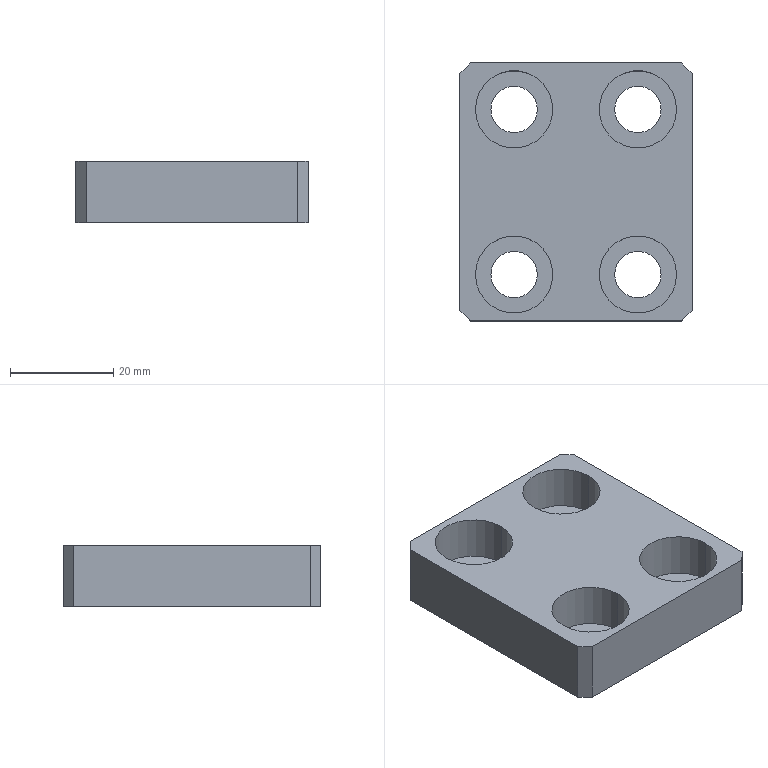Part | SolidWorks | features Chamfer 1, Extrusion 1, HoleWzd 1 | 1 solid | 30 faces | box 45 x 50 x 12 mm | volume 19960 mm3 | cylinder 16 | plane 14 | commonest cylinder face diameters 9 x8 15 x8
STEP:
#1=CARTESIAN_POINT('',(-19.5,16.,3.4));
#2=VERTEX_POINT('',#1);
#3=CARTESIAN_POINT('',(-4.5,16.,3.4));
#4=VERTEX_POINT('',#3);
#5=CARTESIAN_POINT('',(-12.,16.,3.4));
#6=DIRECTION('',(0.,0.,1.));
#7=DIRECTION('',(1.,0.,0.));
#8=AXIS2_PLACEMENT_3D('',#5,#6,#7);
#9=CIRCLE('',#8,7.5);
#10=EDGE_CURVE('',#2,#4,#9,.T.);
#11=ORIENTED_EDGE('',*,*,#10,.F.);
#12=CARTESIAN_POINT('',(-19.5,16.,12.));
#13=VERTEX_POINT('',#12);
#14=CARTESIAN_POINT('',(-19.5,16.,12.));
#15=DIRECTION('',(0.,0.,1.));
#16=VECTOR('',#15,1000.);
#17=LINE('',#14,#16);
#18=EDGE_CURVE('',#2,#13,#17,.T.);
#19=ORIENTED_EDGE('',*,*,#18,.T.);
#20=CARTESIAN_POINT('',(-4.5,16.,12.));
#21=VERTEX_POINT('',#20);
#22=CARTESIAN_POINT('',(-12.,16.,12.));
#23=DIRECTION('',(0.,0.,1.));
#24=DIRECTION('',(1.,0.,0.));
#25=AXIS2_PLACEMENT_3D('',#22,#23,#24);
#26=CIRCLE('',#25,7.5);
#27=EDGE_CURVE('',#13,#21,#26,.T.);
#28=ORIENTED_EDGE('',*,*,#27,.T.);
#29=CARTESIAN_POINT('',(-4.5,16.,12.));
#30=DIRECTION('',(0.,0.,1.));
#31=VECTOR('',#30,1000.);
#32=LINE('',#29,#31);
#33=EDGE_CURVE('',#4,#21,#32,.T.);
#34=ORIENTED_EDGE('',*,*,#33,.F.);
#35=EDGE_LOOP('',(#11,#19,#28,#34));
#36=FACE_OUTER_BOUND('',#35,.T.);
#37=CARTESIAN_POINT('',(-12.,16.,12.));
#38=DIRECTION('',(0.,0.,1.));
#39=DIRECTION('',(1.,0.,0.));
#40=AXIS2_PLACEMENT_3D('',#37,#38,#39);
#41=CYLINDRICAL_SURFACE('',#40,7.5);
#42=ADVANCED_FACE('',(#36),#41,.F.);
#43=CARTESIAN_POINT('',(-16.5,16.,0.));
#44=VERTEX_POINT('',#43);
#45=CARTESIAN_POINT('',(-7.5,16.,0.));
#46=VERTEX_POINT('',#45);
#47=CARTESIAN_POINT('',(-12.,16.,0.));
#48=DIRECTION('',(0.,0.,1.));
#49=DIRECTION('',(1.,0.,0.));
#50=AXIS2_PLACEMENT_3D('',#47,#48,#49);
#51=CIRCLE('',#50,4.5);
#52=EDGE_CURVE('',#44,#46,#51,.T.);
#53=ORIENTED_EDGE('',*,*,#52,.F.);
#54=CARTESIAN_POINT('',(-16.5,16.,3.4));
#55=VERTEX_POINT('',#54);
#56=CARTESIAN_POINT('',(-16.5,16.,12.));
#57=DIRECTION('',(0.,0.,1.));
#58=VECTOR('',#57,1000.);
#59=LINE('',#56,#58);
#60=EDGE_CURVE('',#44,#55,#59,.T.);
#61=ORIENTED_EDGE('',*,*,#60,.T.);
#62=CARTESIAN_POINT('',(-7.5,16.,3.4));
#63=VERTEX_POINT('',#62);
#64=CARTESIAN_POINT('',(-12.,16.,3.4));
#65=DIRECTION('',(0.,0.,1.));
#66=DIRECTION('',(1.,0.,0.));
#67=AXIS2_PLACEMENT_3D('',#64,#65,#66);
#68=CIRCLE('',#67,4.5);
#69=EDGE_CURVE('',#55,#63,#68,.T.);
#70=ORIENTED_EDGE('',*,*,#69,.T.);
#71=CARTESIAN_POINT('',(-7.5,16.,12.));
#72=DIRECTION('',(0.,0.,1.));
#73=VECTOR('',#72,1000.);
#74=LINE('',#71,#73);
#75=EDGE_CURVE('',#46,#63,#74,.T.);
#76=ORIENTED_EDGE('',*,*,#75,.F.);
#77=EDGE_LOOP('',(#53,#61,#70,#76));
#78=FACE_OUTER_BOUND('',#77,.T.);
#79=CARTESIAN_POINT('',(-12.,16.,12.));
#80=DIRECTION('',(0.,0.,1.));
#81=DIRECTION('',(1.,0.,0.));
#82=AXIS2_PLACEMENT_3D('',#79,#80,#81);
#83=CYLINDRICAL_SURFACE('',#82,4.5);
#84=ADVANCED_FACE('',(#78),#83,.F.);
#85=CARTESIAN_POINT('',(4.5,16.,3.4));
#86=VERTEX_POINT('',#85);
#87=CARTESIAN_POINT('',(19.5,16.,3.4));
#88=VERTEX_POINT('',#87);
#89=CARTESIAN_POINT('',(12.,16.,3.4));
#90=DIRECTION('',(0.,0.,1.));
#91=DIRECTION('',(1.,0.,0.));
#92=AXIS2_PLACEMENT_3D('',#89,#90,#91);
#93=CIRCLE('',#92,7.5);
#94=EDGE_CURVE('',#86,#88,#93,.T.);
#95=ORIENTED_EDGE('',*,*,#94,.F.);
#96=CARTESIAN_POINT('',(4.5,16.,12.));
#97=VERTEX_POINT('',#96);
#98=CARTESIAN_POINT('',(4.5,16.,12.));
#99=DIRECTION('',(0.,0.,1.));
#100=VECTOR('',#99,1000.);
#101=LINE('',#98,#100);
#102=EDGE_CURVE('',#86,#97,#101,.T.);
#103=ORIENTED_EDGE('',*,*,#102,.T.);
#104=CARTESIAN_POINT('',(19.5,16.,12.));
#105=VERTEX_POINT('',#104);
#106=CARTESIAN_POINT('',(12.,16.,12.));
#107=DIRECTION('',(0.,0.,1.));
#108=DIRECTION('',(1.,0.,0.));
#109=AXIS2_PLACEMENT_3D('',#106,#107,#108);
#110=CIRCLE('',#109,7.5);
#111=EDGE_CURVE('',#97,#105,#110,.T.);
#112=ORIENTED_EDGE('',*,*,#111,.T.);
#113=CARTESIAN_POINT('',(19.5,16.,12.));
#114=DIRECTION('',(0.,0.,1.));
#115=VECTOR('',#114,1000.);
#116=LINE('',#113,#115);
#117=EDGE_CURVE('',#88,#105,#116,.T.);
#118=ORIENTED_EDGE('',*,*,#117,.F.);
#119=EDGE_LOOP('',(#95,#103,#112,#118));
#120=FACE_OUTER_BOUND('',#119,.T.);
#121=CARTESIAN_POINT('',(12.,16.,12.));
#122=DIRECTION('',(0.,0.,1.));
#123=DIRECTION('',(1.,0.,0.));
#124=AXIS2_PLACEMENT_3D('',#121,#122,#123);
#125=CYLINDRICAL_SURFACE('',#124,7.5);
#126=ADVANCED_FACE('',(#120),#125,.F.);
#127=CARTESIAN_POINT('',(7.5,16.,0.));
#128=VERTEX_POINT('',#127);
#129=CARTESIAN_POINT('',(16.5,16.,0.));
#130=VERTEX_POINT('',#129);
#131=CARTESIAN_POINT('',(12.,16.,0.));
#132=DIRECTION('',(0.,0.,1.));
#133=DIRECTION('',(1.,0.,0.));
#134=AXIS2_PLACEMENT_3D('',#131,#132,#133);
#135=CIRCLE('',#134,4.5);
#136=EDGE_CURVE('',#128,#130,#135,.T.);
#137=ORIENTED_EDGE('',*,*,#136,.F.);
#138=CARTESIAN_POINT('',(7.5,16.,3.4));
#139=VERTEX_POINT('',#138);
#140=CARTESIAN_POINT('',(7.5,16.,12.));
#141=DIRECTION('',(0.,0.,1.));
#142=VECTOR('',#141,1000.);
#143=LINE('',#140,#142);
#144=EDGE_CURVE('',#128,#139,#143,.T.);
#145=ORIENTED_EDGE('',*,*,#144,.T.);
#146=CARTESIAN_POINT('',(16.5,16.,3.4));
#147=VERTEX_POINT('',#146);
#148=CARTESIAN_POINT('',(12.,16.,3.4));
#149=DIRECTION('',(0.,0.,1.));
#150=DIRECTION('',(1.,0.,0.));
#151=AXIS2_PLACEMENT_3D('',#148,#149,#150);
#152=CIRCLE('',#151,4.5);
#153=EDGE_CURVE('',#139,#147,#152,.T.);
#154=ORIENTED_EDGE('',*,*,#153,.T.);
#155=CARTESIAN_POINT('',(16.5,16.,12.));
#156=DIRECTION('',(0.,0.,1.));
#157=VECTOR('',#156,1000.);
#158=LINE('',#155,#157);
#159=EDGE_CURVE('',#130,#147,#158,.T.);
#160=ORIENTED_EDGE('',*,*,#159,.F.);
#161=EDGE_LOOP('',(#137,#145,#154,#160));
#162=FACE_OUTER_BOUND('',#161,.T.);
#163=CARTESIAN_POINT('',(12.,16.,12.));
#164=DIRECTION('',(0.,0.,1.));
#165=DIRECTION('',(1.,0.,0.));
#166=AXIS2_PLACEMENT_3D('',#163,#164,#165);
#167=CYLINDRICAL_SURFACE('',#166,4.5);
#168=ADVANCED_FACE('',(#162),#167,.F.);
#169=CARTESIAN_POINT('',(4.5,-16.,3.4));
#170=VERTEX_POINT('',#169);
#171=CARTESIAN_POINT('',(19.5,-16.,3.4));
#172=VERTEX_POINT('',#171);
#173=CARTESIAN_POINT('',(12.,-16.,3.4));
#174=DIRECTION('',(0.,0.,1.));
#175=DIRECTION('',(1.,0.,0.));
#176=AXIS2_PLACEMENT_3D('',#173,#174,#175);
#177=CIRCLE('',#176,7.5);
#178=EDGE_CURVE('',#170,#172,#177,.T.);
#179=ORIENTED_EDGE('',*,*,#178,.F.);
#180=CARTESIAN_POINT('',(4.5,-16.,12.));
#181=VERTEX_POINT('',#180);
#182=CARTESIAN_POINT('',(4.5,-16.,12.));
#183=DIRECTION('',(0.,0.,1.));
#184=VECTOR('',#183,1000.);
#185=LINE('',#182,#184);
#186=EDGE_CURVE('',#170,#181,#185,.T.);
#187=ORIENTED_EDGE('',*,*,#186,.T.);
#188=CARTESIAN_POINT('',(19.5,-16.,12.));
#189=VERTEX_POINT('',#188);
#190=CARTESIAN_POINT('',(12.,-16.,12.));
#191=DIRECTION('',(0.,0.,1.));
#192=DIRECTION('',(1.,0.,0.));
#193=AXIS2_PLACEMENT_3D('',#190,#191,#192);
#194=CIRCLE('',#193,7.5);
#195=EDGE_CURVE('',#181,#189,#194,.T.);
#196=ORIENTED_EDGE('',*,*,#195,.T.);
#197=CARTESIAN_POINT('',(19.5,-16.,12.));
#198=DIRECTION('',(0.,0.,1.));
#199=VECTOR('',#198,1000.);
#200=LINE('',#197,#199);
#201=EDGE_CURVE('',#172,#189,#200,.T.);
#202=ORIENTED_EDGE('',*,*,#201,.F.);
#203=EDGE_LOOP('',(#179,#187,#196,#202));
#204=FACE_OUTER_BOUND('',#203,.T.);
#205=CARTESIAN_POINT('',(12.,-16.,12.));
#206=DIRECTION('',(0.,0.,1.));
#207=DIRECTION('',(1.,0.,0.));
#208=AXIS2_PLACEMENT_3D('',#205,#206,#207);
#209=CYLINDRICAL_SURFACE('',#208,7.5);
#210=ADVANCED_FACE('',(#204),#209,.F.);
#211=CARTESIAN_POINT('',(7.5,-16.,0.));
#212=VERTEX_POINT('',#211);
#213=CARTESIAN_POINT('',(16.5,-16.,0.));
#214=VERTEX_POINT('',#213);
#215=CARTESIAN_POINT('',(12.,-16.,0.));
#216=DIRECTION('',(0.,0.,1.));
#217=DIRECTION('',(1.,0.,0.));
#218=AXIS2_PLACEMENT_3D('',#215,#216,#217);
#219=CIRCLE('',#218,4.5);
#220=EDGE_CURVE('',#212,#214,#219,.T.);
#221=ORIENTED_EDGE('',*,*,#220,.F.);
#222=CARTESIAN_POINT('',(7.5,-16.,3.4));
#223=VERTEX_POINT('',#222);
#224=CARTESIAN_POINT('',(7.5,-16.,12.));
#225=DIRECTION('',(0.,0.,1.));
#226=VECTOR('',#225,1000.);
#227=LINE('',#224,#226);
#228=EDGE_CURVE('',#212,#223,#227,.T.);
#229=ORIENTED_EDGE('',*,*,#228,.T.);
#230=CARTESIAN_POINT('',(16.5,-16.,3.4));
#231=VERTEX_POINT('',#230);
#232=CARTESIAN_POINT('',(12.,-16.,3.4));
#233=DIRECTION('',(0.,0.,1.));
#234=DIRECTION('',(1.,0.,0.));
#235=AXIS2_PLACEMENT_3D('',#232,#233,#234);
#236=CIRCLE('',#235,4.5);
#237=EDGE_CURVE('',#223,#231,#236,.T.);
#238=ORIENTED_EDGE('',*,*,#237,.T.);
#239=CARTESIAN_POINT('',(16.5,-16.,12.));
#240=DIRECTION('',(0.,0.,1.));
#241=VECTOR('',#240,1000.);
#242=LINE('',#239,#241);
#243=EDGE_CURVE('',#214,#231,#242,.T.);
#244=ORIENTED_EDGE('',*,*,#243,.F.);
#245=EDGE_LOOP('',(#221,#229,#238,#244));
#246=FACE_OUTER_BOUND('',#245,.T.);
#247=CARTESIAN_POINT('',(12.,-16.,12.));
#248=DIRECTION('',(0.,0.,1.));
#249=DIRECTION('',(1.,0.,0.));
#250=AXIS2_PLACEMENT_3D('',#247,#248,#249);
#251=CYLINDRICAL_SURFACE('',#250,4.5);
#252=ADVANCED_FACE('',(#246),#251,.F.);
#253=CARTESIAN_POINT('',(-19.5,-16.,3.4));
#254=VERTEX_POINT('',#253);
#255=CARTESIAN_POINT('',(-4.5,-16.,3.4));
#256=VERTEX_POINT('',#255);
#257=CARTESIAN_POINT('',(-12.,-16.,3.4));
#258=DIRECTION('',(0.,0.,1.));
#259=DIRECTION('',(1.,0.,0.));
#260=AXIS2_PLACEMENT_3D('',#257,#258,#259);
#261=CIRCLE('',#260,7.5);
#262=EDGE_CURVE('',#254,#256,#261,.T.);
#263=ORIENTED_EDGE('',*,*,#262,.F.);
#264=CARTESIAN_POINT('',(-19.5,-16.,12.));
#265=VERTEX_POINT('',#264);
#266=CARTESIAN_POINT('',(-19.5,-16.,12.));
#267=DIRECTION('',(0.,0.,1.));
#268=VECTOR('',#267,1000.);
#269=LINE('',#266,#268);
#270=EDGE_CURVE('',#254,#265,#269,.T.);
#271=ORIENTED_EDGE('',*,*,#270,.T.);
#272=CARTESIAN_POINT('',(-4.5,-16.,12.));
#273=VERTEX_POINT('',#272);
#274=CARTESIAN_POINT('',(-12.,-16.,12.));
#275=DIRECTION('',(0.,0.,1.));
#276=DIRECTION('',(1.,0.,0.));
#277=AXIS2_PLACEMENT_3D('',#274,#275,#276);
#278=CIRCLE('',#277,7.5);
#279=EDGE_CURVE('',#265,#273,#278,.T.);
#280=ORIENTED_EDGE('',*,*,#279,.T.);
#281=CARTESIAN_POINT('',(-4.5,-16.,12.));
#282=DIRECTION('',(0.,0.,1.));
#283=VECTOR('',#282,1000.);
#284=LINE('',#281,#283);
#285=EDGE_CURVE('',#256,#273,#284,.T.);
#286=ORIENTED_EDGE('',*,*,#285,.F.);
#287=EDGE_LOOP('',(#263,#271,#280,#286));
#288=FACE_OUTER_BOUND('',#287,.T.);
#289=CARTESIAN_POINT('',(-12.,-16.,12.));
#290=DIRECTION('',(0.,0.,1.));
#291=DIRECTION('',(1.,0.,0.));
#292=AXIS2_PLACEMENT_3D('',#289,#290,#291);
#293=CYLINDRICAL_SURFACE('',#292,7.5);
#294=ADVANCED_FACE('',(#288),#293,.F.);
#295=CARTESIAN_POINT('',(-16.5,-16.,0.));
#296=VERTEX_POINT('',#295);
#297=CARTESIAN_POINT('',(-7.5,-16.,0.));
#298=VERTEX_POINT('',#297);
#299=CARTESIAN_POINT('',(-12.,-16.,0.));
#300=DIRECTION('',(0.,0.,1.));
#301=DIRECTION('',(1.,0.,0.));
#302=AXIS2_PLACEMENT_3D('',#299,#300,#301);
#303=CIRCLE('',#302,4.5);
#304=EDGE_CURVE('',#296,#298,#303,.T.);
#305=ORIENTED_EDGE('',*,*,#304,.F.);
#306=CARTESIAN_POINT('',(-16.5,-16.,3.4));
#307=VERTEX_POINT('',#306);
#308=CARTESIAN_POINT('',(-16.5,-16.,12.));
#309=DIRECTION('',(0.,0.,1.));
#310=VECTOR('',#309,1000.);
#311=LINE('',#308,#310);
#312=EDGE_CURVE('',#296,#307,#311,.T.);
#313=ORIENTED_EDGE('',*,*,#312,.T.);
#314=CARTESIAN_POINT('',(-7.5,-16.,3.4));
#315=VERTEX_POINT('',#314);
#316=CARTESIAN_POINT('',(-12.,-16.,3.4));
#317=DIRECTION('',(0.,0.,1.));
#318=DIRECTION('',(1.,0.,0.));
#319=AXIS2_PLACEMENT_3D('',#316,#317,#318);
#320=CIRCLE('',#319,4.5);
#321=EDGE_CURVE('',#307,#315,#320,.T.);
#322=ORIENTED_EDGE('',*,*,#321,.T.);
#323=CARTESIAN_POINT('',(-7.5,-16.,12.));
#324=DIRECTION('',(0.,0.,1.));
#325=VECTOR('',#324,1000.);
#326=LINE('',#323,#325);
#327=EDGE_CURVE('',#298,#315,#326,.T.);
#328=ORIENTED_EDGE('',*,*,#327,.F.);
#329=EDGE_LOOP('',(#305,#313,#322,#328));
#330=FACE_OUTER_BOUND('',#329,.T.);
#331=CARTESIAN_POINT('',(-12.,-16.,12.));
#332=DIRECTION('',(0.,0.,1.));
#333=DIRECTION('',(1.,0.,0.));
#334=AXIS2_PLACEMENT_3D('',#331,#332,#333);
#335=CYLINDRICAL_SURFACE('',#334,4.5);
#336=ADVANCED_FACE('',(#330),#335,.F.);
#337=CARTESIAN_POINT('',(22.5,-23.,12.));
#338=VERTEX_POINT('',#337);
#339=CARTESIAN_POINT('',(22.5,23.,12.));
#340=VERTEX_POINT('',#339);
#341=CARTESIAN_POINT('',(22.5,25.,12.));
#342=DIRECTION('',(0.,1.,0.));
#343=VECTOR('',#342,1000.);
#344=LINE('',#341,#343);
#345=EDGE_CURVE('',#338,#340,#344,.T.);
#346=ORIENTED_EDGE('',*,*,#345,.F.);
#347=CARTESIAN_POINT('',(22.5,-23.,0.));
#348=VERTEX_POINT('',#347);
#349=CARTESIAN_POINT('',(22.5,-23.,12.));
#350=DIRECTION('',(0.,0.,-1.));
#351=VECTOR('',#350,1000.);
#352=LINE('',#349,#351);
#353=EDGE_CURVE('',#338,#348,#352,.T.);
#354=ORIENTED_EDGE('',*,*,#353,.T.);
#355=CARTESIAN_POINT('',(22.5,23.,0.));
#356=VERTEX_POINT('',#355);
#357=CARTESIAN_POINT('',(22.5,25.,0.));
#358=DIRECTION('',(0.,1.,0.));
#359=VECTOR('',#358,1000.);
#360=LINE('',#357,#359);
#361=EDGE_CURVE('',#348,#356,#360,.T.);
#362=ORIENTED_EDGE('',*,*,#361,.T.);
#363=CARTESIAN_POINT('',(22.5,23.,12.));
#364=DIRECTION('',(0.,0.,1.));
#365=VECTOR('',#364,1000.);
#366=LINE('',#363,#365);
#367=EDGE_CURVE('',#356,#340,#366,.T.);
#368=ORIENTED_EDGE('',*,*,#367,.T.);
#369=EDGE_LOOP('',(#346,#354,#362,#368));
#370=FACE_OUTER_BOUND('',#369,.T.);
#371=CARTESIAN_POINT('',(22.5,25.,12.));
#372=DIRECTION('',(-1.,0.,0.));
#373=DIRECTION('',(0.,-1.,0.));
#374=AXIS2_PLACEMENT_3D('',#371,#372,#373);
#375=PLANE('',#374);
#376=ADVANCED_FACE('',(#370),#375,.F.);
#377=CARTESIAN_POINT('',(20.5,25.,12.));
#378=VERTEX_POINT('',#377);
#379=CARTESIAN_POINT('',(-20.5,25.,12.));
#380=VERTEX_POINT('',#379);
#381=CARTESIAN_POINT('',(-22.5,25.,12.));
#382=DIRECTION('',(-1.,0.,0.));
#383=VECTOR('',#382,1000.);
#384=LINE('',#381,#383);
#385=EDGE_CURVE('',#378,#380,#384,.T.);
#386=ORIENTED_EDGE('',*,*,#385,.F.);
#387=CARTESIAN_POINT('',(20.5,25.,0.));
#388=VERTEX_POINT('',#387);
#389=CARTESIAN_POINT('',(20.5,25.,12.));
#390=DIRECTION('',(0.,0.,-1.));
#391=VECTOR('',#390,1000.);
#392=LINE('',#389,#391);
#393=EDGE_CURVE('',#378,#388,#392,.T.);
#394=ORIENTED_EDGE('',*,*,#393,.T.);
#395=CARTESIAN_POINT('',(-20.5,25.,0.));
#396=VERTEX_POINT('',#395);
#397=CARTESIAN_POINT('',(-22.5,25.,0.));
#398=DIRECTION('',(-1.,0.,0.));
#399=VECTOR('',#398,1000.);
#400=LINE('',#397,#399);
#401=EDGE_CURVE('',#388,#396,#400,.T.);
#402=ORIENTED_EDGE('',*,*,#401,.T.);
#403=CARTESIAN_POINT('',(-20.5,25.,12.));
#404=DIRECTION('',(0.,0.,1.));
#405=VECTOR('',#404,1000.);
#406=LINE('',#403,#405);
#407=EDGE_CURVE('',#396,#380,#406,.T.);
#408=ORIENTED_EDGE('',*,*,#407,.T.);
#409=EDGE_LOOP('',(#386,#394,#402,#408));
#410=FACE_OUTER_BOUND('',#409,.T.);
#411=CARTESIAN_POINT('',(-22.5,25.,12.));
#412=DIRECTION('',(0.,-1.,0.));
#413=DIRECTION('',(0.,0.,-1.));
#414=AXIS2_PLACEMENT_3D('',#411,#412,#413);
#415=PLANE('',#414);
#416=ADVANCED_FACE('',(#410),#415,.F.);
#417=CARTESIAN_POINT('',(-22.5,23.,0.));
#418=VERTEX_POINT('',#417);
#419=CARTESIAN_POINT('',(-22.5,-23.,0.));
#420=VERTEX_POINT('',#419);
#421=CARTESIAN_POINT('',(-22.5,25.,0.));
#422=DIRECTION('',(0.,-1.,0.));
#423=VECTOR('',#422,1000.);
#424=LINE('',#421,#423);
#425=EDGE_CURVE('',#418,#420,#424,.T.);
#426=ORIENTED_EDGE('',*,*,#425,.T.);
#427=CARTESIAN_POINT('',(-22.5,-23.,12.));
#428=VERTEX_POINT('',#427);
#429=CARTESIAN_POINT('',(-22.5,-23.,12.));
#430=DIRECTION('',(0.,0.,1.));
#431=VECTOR('',#430,1000.);
#432=LINE('',#429,#431);
#433=EDGE_CURVE('',#420,#428,#432,.T.);
#434=ORIENTED_EDGE('',*,*,#433,.T.);
#435=CARTESIAN_POINT('',(-22.5,23.,12.));
#436=VERTEX_POINT('',#435);
#437=CARTESIAN_POINT('',(-22.5,25.,12.));
#438=DIRECTION('',(0.,-1.,0.));
#439=VECTOR('',#438,1000.);
#440=LINE('',#437,#439);
#441=EDGE_CURVE('',#436,#428,#440,.T.);
#442=ORIENTED_EDGE('',*,*,#441,.F.);
#443=CARTESIAN_POINT('',(-22.5,23.,12.));
#444=DIRECTION('',(0.,0.,-1.));
#445=VECTOR('',#444,1000.);
#446=LINE('',#443,#445);
#447=EDGE_CURVE('',#436,#418,#446,.T.);
#448=ORIENTED_EDGE('',*,*,#447,.T.);
#449=EDGE_LOOP('',(#426,#434,#442,#448));
#450=FACE_OUTER_BOUND('',#449,.T.);
#451=CARTESIAN_POINT('',(-22.5,25.,12.));
#452=DIRECTION('',(1.,0.,0.));
#453=DIRECTION('',(0.,1.,0.));
#454=AXIS2_PLACEMENT_3D('',#451,#452,#453);
#455=PLANE('',#454);
#456=ADVANCED_FACE('',(#450),#455,.F.);
#457=CARTESIAN_POINT('',(-20.5,-25.,0.));
#458=VERTEX_POINT('',#457);
#459=CARTESIAN_POINT('',(20.5,-25.,0.));
#460=VERTEX_POINT('',#459);
#461=CARTESIAN_POINT('',(-22.5,-25.,0.));
#462=DIRECTION('',(1.,0.,0.));
#463=VECTOR('',#462,1000.);
#464=LINE('',#461,#463);
#465=EDGE_CURVE('',#458,#460,#464,.T.);
#466=ORIENTED_EDGE('',*,*,#465,.T.);
#467=CARTESIAN_POINT('',(20.5,-25.,12.));
#468=VERTEX_POINT('',#467);
#469=CARTESIAN_POINT('',(20.5,-25.,12.));
#470=DIRECTION('',(0.,0.,1.));
#471=VECTOR('',#470,1000.);
#472=LINE('',#469,#471);
#473=EDGE_CURVE('',#460,#468,#472,.T.);
#474=ORIENTED_EDGE('',*,*,#473,.T.);
#475=CARTESIAN_POINT('',(-20.5,-25.,12.));
#476=VERTEX_POINT('',#475);
#477=CARTESIAN_POINT('',(-22.5,-25.,12.));
#478=DIRECTION('',(1.,0.,0.));
#479=VECTOR('',#478,1000.);
#480=LINE('',#477,#479);
#481=EDGE_CURVE('',#476,#468,#480,.T.);
#482=ORIENTED_EDGE('',*,*,#481,.F.);
#483=CARTESIAN_POINT('',(-20.5,-25.,12.));
#484=DIRECTION('',(0.,0.,-1.));
#485=VECTOR('',#484,1000.);
#486=LINE('',#483,#485);
#487=EDGE_CURVE('',#476,#458,#486,.T.);
#488=ORIENTED_EDGE('',*,*,#487,.T.);
#489=EDGE_LOOP('',(#466,#474,#482,#488));
#490=FACE_OUTER_BOUND('',#489,.T.);
#491=CARTESIAN_POINT('',(-22.5,-25.,12.));
#492=DIRECTION('',(0.,1.,0.));
#493=DIRECTION('',(0.,0.,1.));
#494=AXIS2_PLACEMENT_3D('',#491,#492,#493);
#495=PLANE('',#494);
#496=ADVANCED_FACE('',(#490),#495,.F.);
#497=CARTESIAN_POINT('',(-12.,16.,12.));
#498=DIRECTION('',(0.,0.,1.));
#499=DIRECTION('',(1.,0.,0.));
#500=AXIS2_PLACEMENT_3D('',#497,#498,#499);
#501=CIRCLE('',#500,7.5);
#502=EDGE_CURVE('',#21,#13,#501,.T.);
#503=ORIENTED_EDGE('',*,*,#502,.F.);
#504=ORIENTED_EDGE('',*,*,#27,.F.);
#505=EDGE_LOOP('',(#503,#504));
#506=FACE_BOUND('',#505,.T.);
#507=CARTESIAN_POINT('',(12.,16.,12.));
#508=DIRECTION('',(0.,0.,1.));
#509=DIRECTION('',(1.,0.,0.));
#510=AXIS2_PLACEMENT_3D('',#507,#508,#509);
#511=CIRCLE('',#510,7.5);
#512=EDGE_CURVE('',#105,#97,#511,.T.);
#513=ORIENTED_EDGE('',*,*,#512,.F.);
#514=ORIENTED_EDGE('',*,*,#111,.F.);
#515=EDGE_LOOP('',(#513,#514));
#516=FACE_BOUND('',#515,.T.);
#517=CARTESIAN_POINT('',(12.,-16.,12.));
#518=DIRECTION('',(0.,0.,1.));
#519=DIRECTION('',(1.,0.,0.));
#520=AXIS2_PLACEMENT_3D('',#517,#518,#519);
#521=CIRCLE('',#520,7.5);
#522=EDGE_CURVE('',#189,#181,#521,.T.);
#523=ORIENTED_EDGE('',*,*,#522,.F.);
#524=ORIENTED_EDGE('',*,*,#195,.F.);
#525=EDGE_LOOP('',(#523,#524));
#526=FACE_BOUND('',#525,.T.);
#527=CARTESIAN_POINT('',(-12.,-16.,12.));
#528=DIRECTION('',(0.,0.,1.));
#529=DIRECTION('',(1.,0.,0.));
#530=AXIS2_PLACEMENT_3D('',#527,#528,#529);
#531=CIRCLE('',#530,7.5);
#532=EDGE_CURVE('',#273,#265,#531,.T.);
#533=ORIENTED_EDGE('',*,*,#532,.F.);
#534=ORIENTED_EDGE('',*,*,#279,.F.);
#535=EDGE_LOOP('',(#533,#534));
#536=FACE_BOUND('',#535,.T.);
#537=ORIENTED_EDGE('',*,*,#481,.T.);
#538=CARTESIAN_POINT('',(22.75,-22.75,12.));
#539=DIRECTION('',(0.7071,0.7071,0.));
#540=VECTOR('',#539,1000.);
#541=LINE('',#538,#540);
#542=EDGE_CURVE('',#468,#338,#541,.T.);
#543=ORIENTED_EDGE('',*,*,#542,.T.);
#544=ORIENTED_EDGE('',*,*,#345,.T.);
#545=CARTESIAN_POINT('',(22.75,22.75,12.));
#546=DIRECTION('',(-0.7071,0.7071,0.));
#547=VECTOR('',#546,1000.);
#548=LINE('',#545,#547);
#549=EDGE_CURVE('',#340,#378,#548,.T.);
#550=ORIENTED_EDGE('',*,*,#549,.T.);
#551=ORIENTED_EDGE('',*,*,#385,.T.);
#552=CARTESIAN_POINT('',(-22.75,22.75,12.));
#553=DIRECTION('',(-0.7071,-0.7071,0.));
#554=VECTOR('',#553,1000.);
#555=LINE('',#552,#554);
#556=EDGE_CURVE('',#380,#436,#555,.T.);
#557=ORIENTED_EDGE('',*,*,#556,.T.);
#558=ORIENTED_EDGE('',*,*,#441,.T.);
#559=CARTESIAN_POINT('',(-22.75,-22.75,12.));
#560=DIRECTION('',(0.7071,-0.7071,0.));
#561=VECTOR('',#560,1000.);
#562=LINE('',#559,#561);
#563=EDGE_CURVE('',#428,#476,#562,.T.);
#564=ORIENTED_EDGE('',*,*,#563,.T.);
#565=EDGE_LOOP('',(#537,#543,#544,#550,#551,#557,#558,#564));
#566=FACE_OUTER_BOUND('',#565,.T.);
#567=CARTESIAN_POINT('',(0.,0.,12.));
#568=DIRECTION('',(0.,0.,1.));
#569=DIRECTION('',(1.,0.,0.));
#570=AXIS2_PLACEMENT_3D('',#567,#568,#569);
#571=PLANE('',#570);
#572=ADVANCED_FACE('',(#506,#516,#526,#536,#566),#571,.T.);
#573=CARTESIAN_POINT('',(-12.,16.,0.));
#574=DIRECTION('',(0.,0.,1.));
#575=DIRECTION('',(1.,0.,0.));
#576=AXIS2_PLACEMENT_3D('',#573,#574,#575);
#577=CIRCLE('',#576,4.5);
#578=EDGE_CURVE('',#46,#44,#577,.T.);
#579=ORIENTED_EDGE('',*,*,#578,.T.);
#580=ORIENTED_EDGE('',*,*,#52,.T.);
#581=EDGE_LOOP('',(#579,#580));
#582=FACE_BOUND('',#581,.T.);
#583=CARTESIAN_POINT('',(12.,16.,0.));
#584=DIRECTION('',(0.,0.,1.));
#585=DIRECTION('',(1.,0.,0.));
#586=AXIS2_PLACEMENT_3D('',#583,#584,#585);
#587=CIRCLE('',#586,4.5);
#588=EDGE_CURVE('',#130,#128,#587,.T.);
#589=ORIENTED_EDGE('',*,*,#588,.T.);
#590=ORIENTED_EDGE('',*,*,#136,.T.);
#591=EDGE_LOOP('',(#589,#590));
#592=FACE_BOUND('',#591,.T.);
#593=CARTESIAN_POINT('',(12.,-16.,0.));
#594=DIRECTION('',(0.,0.,1.));
#595=DIRECTION('',(1.,0.,0.));
#596=AXIS2_PLACEMENT_3D('',#593,#594,#595);
#597=CIRCLE('',#596,4.5);
#598=EDGE_CURVE('',#214,#212,#597,.T.);
#599=ORIENTED_EDGE('',*,*,#598,.T.);
#600=ORIENTED_EDGE('',*,*,#220,.T.);
#601=EDGE_LOOP('',(#599,#600));
#602=FACE_BOUND('',#601,.T.);
#603=CARTESIAN_POINT('',(-12.,-16.,0.));
#604=DIRECTION('',(0.,0.,1.));
#605=DIRECTION('',(1.,0.,0.));
#606=AXIS2_PLACEMENT_3D('',#603,#604,#605);
#607=CIRCLE('',#606,4.5);
#608=EDGE_CURVE('',#298,#296,#607,.T.);
#609=ORIENTED_EDGE('',*,*,#608,.T.);
#610=ORIENTED_EDGE('',*,*,#304,.T.);
#611=EDGE_LOOP('',(#609,#610));
#612=FACE_BOUND('',#611,.T.);
#613=ORIENTED_EDGE('',*,*,#361,.F.);
#614=CARTESIAN_POINT('',(22.5,-23.,0.));
#615=DIRECTION('',(-0.7071,-0.7071,0.));
#616=VECTOR('',#615,1000.);
#617=LINE('',#614,#616);
#618=EDGE_CURVE('',#348,#460,#617,.T.);
#619=ORIENTED_EDGE('',*,*,#618,.T.);
#620=ORIENTED_EDGE('',*,*,#465,.F.);
#621=CARTESIAN_POINT('',(-20.5,-25.,0.));
#622=DIRECTION('',(-0.7071,0.7071,0.));
#623=VECTOR('',#622,1000.);
#624=LINE('',#621,#623);
#625=EDGE_CURVE('',#458,#420,#624,.T.);
#626=ORIENTED_EDGE('',*,*,#625,.T.);
#627=ORIENTED_EDGE('',*,*,#425,.F.);
#628=CARTESIAN_POINT('',(-22.5,23.,0.));
#629=DIRECTION('',(0.7071,0.7071,0.));
#630=VECTOR('',#629,1000.);
#631=LINE('',#628,#630);
#632=EDGE_CURVE('',#418,#396,#631,.T.);
#633=ORIENTED_EDGE('',*,*,#632,.T.);
#634=ORIENTED_EDGE('',*,*,#401,.F.);
#635=CARTESIAN_POINT('',(20.5,25.,0.));
#636=DIRECTION('',(0.7071,-0.7071,0.));
#637=VECTOR('',#636,1000.);
#638=LINE('',#635,#637);
#639=EDGE_CURVE('',#388,#356,#638,.T.);
#640=ORIENTED_EDGE('',*,*,#639,.T.);
#641=EDGE_LOOP('',(#613,#619,#620,#626,#627,#633,#634,#640));
#642=FACE_OUTER_BOUND('',#641,.T.);
#643=CARTESIAN_POINT('',(0.,0.,0.));
#644=DIRECTION('',(0.,0.,1.));
#645=DIRECTION('',(1.,0.,0.));
#646=AXIS2_PLACEMENT_3D('',#643,#644,#645);
#647=PLANE('',#646);
#648=ADVANCED_FACE('',(#582,#592,#602,#612,#642),#647,.F.);
#649=ORIENTED_EDGE('',*,*,#312,.F.);
#650=ORIENTED_EDGE('',*,*,#608,.F.);
#651=ORIENTED_EDGE('',*,*,#327,.T.);
#652=CARTESIAN_POINT('',(-12.,-16.,3.4));
#653=DIRECTION('',(0.,0.,1.));
#654=DIRECTION('',(1.,0.,0.));
#655=AXIS2_PLACEMENT_3D('',#652,#653,#654);
#656=CIRCLE('',#655,4.5);
#657=EDGE_CURVE('',#315,#307,#656,.T.);
#658=ORIENTED_EDGE('',*,*,#657,.T.);
#659=EDGE_LOOP('',(#649,#650,#651,#658));
#660=FACE_OUTER_BOUND('',#659,.T.);
#661=CARTESIAN_POINT('',(-12.,-16.,12.));
#662=DIRECTION('',(0.,0.,1.));
#663=DIRECTION('',(1.,0.,0.));
#664=AXIS2_PLACEMENT_3D('',#661,#662,#663);
#665=CYLINDRICAL_SURFACE('',#664,4.5);
#666=ADVANCED_FACE('',(#660),#665,.F.);
#667=ORIENTED_EDGE('',*,*,#657,.F.);
#668=ORIENTED_EDGE('',*,*,#321,.F.);
#669=EDGE_LOOP('',(#667,#668));
#670=FACE_BOUND('',#669,.T.);
#671=CARTESIAN_POINT('',(-12.,-16.,3.4));
#672=DIRECTION('',(0.,0.,1.));
#673=DIRECTION('',(1.,0.,0.));
#674=AXIS2_PLACEMENT_3D('',#671,#672,#673);
#675=CIRCLE('',#674,7.5);
#676=EDGE_CURVE('',#256,#254,#675,.T.);
#677=ORIENTED_EDGE('',*,*,#676,.T.);
#678=ORIENTED_EDGE('',*,*,#262,.T.);
#679=EDGE_LOOP('',(#677,#678));
#680=FACE_OUTER_BOUND('',#679,.T.);
#681=CARTESIAN_POINT('',(-7.5,-16.,3.4));
#682=DIRECTION('',(0.,0.,-1.));
#683=DIRECTION('',(-1.,0.,0.));
#684=AXIS2_PLACEMENT_3D('',#681,#682,#683);
#685=PLANE('',#684);
#686=ADVANCED_FACE('',(#670,#680),#685,.F.);
#687=ORIENTED_EDGE('',*,*,#270,.F.);
#688=ORIENTED_EDGE('',*,*,#676,.F.);
#689=ORIENTED_EDGE('',*,*,#285,.T.);
#690=ORIENTED_EDGE('',*,*,#532,.T.);
#691=EDGE_LOOP('',(#687,#688,#689,#690));
#692=FACE_OUTER_BOUND('',#691,.T.);
#693=CARTESIAN_POINT('',(-12.,-16.,12.));
#694=DIRECTION('',(0.,0.,1.));
#695=DIRECTION('',(1.,0.,0.));
#696=AXIS2_PLACEMENT_3D('',#693,#694,#695);
#697=CYLINDRICAL_SURFACE('',#696,7.5);
#698=ADVANCED_FACE('',(#692),#697,.F.);
#699=ORIENTED_EDGE('',*,*,#228,.F.);
#700=ORIENTED_EDGE('',*,*,#598,.F.);
#701=ORIENTED_EDGE('',*,*,#243,.T.);
#702=CARTESIAN_POINT('',(12.,-16.,3.4));
#703=DIRECTION('',(0.,0.,1.));
#704=DIRECTION('',(1.,0.,0.));
#705=AXIS2_PLACEMENT_3D('',#702,#703,#704);
#706=CIRCLE('',#705,4.5);
#707=EDGE_CURVE('',#231,#223,#706,.T.);
#708=ORIENTED_EDGE('',*,*,#707,.T.);
#709=EDGE_LOOP('',(#699,#700,#701,#708));
#710=FACE_OUTER_BOUND('',#709,.T.);
#711=CARTESIAN_POINT('',(12.,-16.,12.));
#712=DIRECTION('',(0.,0.,1.));
#713=DIRECTION('',(1.,0.,0.));
#714=AXIS2_PLACEMENT_3D('',#711,#712,#713);
#715=CYLINDRICAL_SURFACE('',#714,4.5);
#716=ADVANCED_FACE('',(#710),#715,.F.);
#717=ORIENTED_EDGE('',*,*,#707,.F.);
#718=ORIENTED_EDGE('',*,*,#237,.F.);
#719=EDGE_LOOP('',(#717,#718));
#720=FACE_BOUND('',#719,.T.);
#721=CARTESIAN_POINT('',(12.,-16.,3.4));
#722=DIRECTION('',(0.,0.,1.));
#723=DIRECTION('',(1.,0.,0.));
#724=AXIS2_PLACEMENT_3D('',#721,#722,#723);
#725=CIRCLE('',#724,7.5);
#726=EDGE_CURVE('',#172,#170,#725,.T.);
#727=ORIENTED_EDGE('',*,*,#726,.T.);
#728=ORIENTED_EDGE('',*,*,#178,.T.);
#729=EDGE_LOOP('',(#727,#728));
#730=FACE_OUTER_BOUND('',#729,.T.);
#731=CARTESIAN_POINT('',(16.5,-16.,3.4));
#732=DIRECTION('',(0.,0.,-1.));
#733=DIRECTION('',(-1.,0.,0.));
#734=AXIS2_PLACEMENT_3D('',#731,#732,#733);
#735=PLANE('',#734);
#736=ADVANCED_FACE('',(#720,#730),#735,.F.);
#737=ORIENTED_EDGE('',*,*,#186,.F.);
#738=ORIENTED_EDGE('',*,*,#726,.F.);
#739=ORIENTED_EDGE('',*,*,#201,.T.);
#740=ORIENTED_EDGE('',*,*,#522,.T.);
#741=EDGE_LOOP('',(#737,#738,#739,#740));
#742=FACE_OUTER_BOUND('',#741,.T.);
#743=CARTESIAN_POINT('',(12.,-16.,12.));
#744=DIRECTION('',(0.,0.,1.));
#745=DIRECTION('',(1.,0.,0.));
#746=AXIS2_PLACEMENT_3D('',#743,#744,#745);
#747=CYLINDRICAL_SURFACE('',#746,7.5);
#748=ADVANCED_FACE('',(#742),#747,.F.);
#749=ORIENTED_EDGE('',*,*,#144,.F.);
#750=ORIENTED_EDGE('',*,*,#588,.F.);
#751=ORIENTED_EDGE('',*,*,#159,.T.);
#752=CARTESIAN_POINT('',(12.,16.,3.4));
#753=DIRECTION('',(0.,0.,1.));
#754=DIRECTION('',(1.,0.,0.));
#755=AXIS2_PLACEMENT_3D('',#752,#753,#754);
#756=CIRCLE('',#755,4.5);
#757=EDGE_CURVE('',#147,#139,#756,.T.);
#758=ORIENTED_EDGE('',*,*,#757,.T.);
#759=EDGE_LOOP('',(#749,#750,#751,#758));
#760=FACE_OUTER_BOUND('',#759,.T.);
#761=CARTESIAN_POINT('',(12.,16.,12.));
#762=DIRECTION('',(0.,0.,1.));
#763=DIRECTION('',(1.,0.,0.));
#764=AXIS2_PLACEMENT_3D('',#761,#762,#763);
#765=CYLINDRICAL_SURFACE('',#764,4.5);
#766=ADVANCED_FACE('',(#760),#765,.F.);
#767=ORIENTED_EDGE('',*,*,#757,.F.);
#768=ORIENTED_EDGE('',*,*,#153,.F.);
#769=EDGE_LOOP('',(#767,#768));
#770=FACE_BOUND('',#769,.T.);
#771=CARTESIAN_POINT('',(12.,16.,3.4));
#772=DIRECTION('',(0.,0.,1.));
#773=DIRECTION('',(1.,0.,0.));
#774=AXIS2_PLACEMENT_3D('',#771,#772,#773);
#775=CIRCLE('',#774,7.5);
#776=EDGE_CURVE('',#88,#86,#775,.T.);
#777=ORIENTED_EDGE('',*,*,#776,.T.);
#778=ORIENTED_EDGE('',*,*,#94,.T.);
#779=EDGE_LOOP('',(#777,#778));
#780=FACE_OUTER_BOUND('',#779,.T.);
#781=CARTESIAN_POINT('',(16.5,16.,3.4));
#782=DIRECTION('',(0.,0.,-1.));
#783=DIRECTION('',(-1.,0.,0.));
#784=AXIS2_PLACEMENT_3D('',#781,#782,#783);
#785=PLANE('',#784);
#786=ADVANCED_FACE('',(#770,#780),#785,.F.);
#787=ORIENTED_EDGE('',*,*,#102,.F.);
#788=ORIENTED_EDGE('',*,*,#776,.F.);
#789=ORIENTED_EDGE('',*,*,#117,.T.);
#790=ORIENTED_EDGE('',*,*,#512,.T.);
#791=EDGE_LOOP('',(#787,#788,#789,#790));
#792=FACE_OUTER_BOUND('',#791,.T.);
#793=CARTESIAN_POINT('',(12.,16.,12.));
#794=DIRECTION('',(0.,0.,1.));
#795=DIRECTION('',(1.,0.,0.));
#796=AXIS2_PLACEMENT_3D('',#793,#794,#795);
#797=CYLINDRICAL_SURFACE('',#796,7.5);
#798=ADVANCED_FACE('',(#792),#797,.F.);
#799=ORIENTED_EDGE('',*,*,#60,.F.);
#800=ORIENTED_EDGE('',*,*,#578,.F.);
#801=ORIENTED_EDGE('',*,*,#75,.T.);
#802=CARTESIAN_POINT('',(-12.,16.,3.4));
#803=DIRECTION('',(0.,0.,1.));
#804=DIRECTION('',(1.,0.,0.));
#805=AXIS2_PLACEMENT_3D('',#802,#803,#804);
#806=CIRCLE('',#805,4.5);
#807=EDGE_CURVE('',#63,#55,#806,.T.);
#808=ORIENTED_EDGE('',*,*,#807,.T.);
#809=EDGE_LOOP('',(#799,#800,#801,#808));
#810=FACE_OUTER_BOUND('',#809,.T.);
#811=CARTESIAN_POINT('',(-12.,16.,12.));
#812=DIRECTION('',(0.,0.,1.));
#813=DIRECTION('',(1.,0.,0.));
#814=AXIS2_PLACEMENT_3D('',#811,#812,#813);
#815=CYLINDRICAL_SURFACE('',#814,4.5);
#816=ADVANCED_FACE('',(#810),#815,.F.);
#817=ORIENTED_EDGE('',*,*,#807,.F.);
#818=ORIENTED_EDGE('',*,*,#69,.F.);
#819=EDGE_LOOP('',(#817,#818));
#820=FACE_BOUND('',#819,.T.);
#821=CARTESIAN_POINT('',(-12.,16.,3.4));
#822=DIRECTION('',(0.,0.,1.));
#823=DIRECTION('',(1.,0.,0.));
#824=AXIS2_PLACEMENT_3D('',#821,#822,#823);
#825=CIRCLE('',#824,7.5);
#826=EDGE_CURVE('',#4,#2,#825,.T.);
#827=ORIENTED_EDGE('',*,*,#826,.T.);
#828=ORIENTED_EDGE('',*,*,#10,.T.);
#829=EDGE_LOOP('',(#827,#828));
#830=FACE_OUTER_BOUND('',#829,.T.);
#831=CARTESIAN_POINT('',(-7.5,16.,3.4));
#832=DIRECTION('',(0.,0.,-1.));
#833=DIRECTION('',(-1.,0.,0.));
#834=AXIS2_PLACEMENT_3D('',#831,#832,#833);
#835=PLANE('',#834);
#836=ADVANCED_FACE('',(#820,#830),#835,.F.);
#837=ORIENTED_EDGE('',*,*,#18,.F.);
#838=ORIENTED_EDGE('',*,*,#826,.F.);
#839=ORIENTED_EDGE('',*,*,#33,.T.);
#840=ORIENTED_EDGE('',*,*,#502,.T.);
#841=EDGE_LOOP('',(#837,#838,#839,#840));
#842=FACE_OUTER_BOUND('',#841,.T.);
#843=CARTESIAN_POINT('',(-12.,16.,12.));
#844=DIRECTION('',(0.,0.,1.));
#845=DIRECTION('',(1.,0.,0.));
#846=AXIS2_PLACEMENT_3D('',#843,#844,#845);
#847=CYLINDRICAL_SURFACE('',#846,7.5);
#848=ADVANCED_FACE('',(#842),#847,.F.);
#849=ORIENTED_EDGE('',*,*,#542,.F.);
#850=ORIENTED_EDGE('',*,*,#473,.F.);
#851=ORIENTED_EDGE('',*,*,#618,.F.);
#852=ORIENTED_EDGE('',*,*,#353,.F.);
#853=EDGE_LOOP('',(#849,#850,#851,#852));
#854=FACE_OUTER_BOUND('',#853,.T.);
#855=CARTESIAN_POINT('',(22.5,-23.,12.));
#856=DIRECTION('',(-0.7071,0.7071,0.));
#857=DIRECTION('',(0.,0.,-1.));
#858=AXIS2_PLACEMENT_3D('',#855,#856,#857);
#859=PLANE('',#858);
#860=ADVANCED_FACE('',(#854),#859,.F.);
#861=ORIENTED_EDGE('',*,*,#563,.F.);
#862=ORIENTED_EDGE('',*,*,#433,.F.);
#863=ORIENTED_EDGE('',*,*,#625,.F.);
#864=ORIENTED_EDGE('',*,*,#487,.F.);
#865=EDGE_LOOP('',(#861,#862,#863,#864));
#866=FACE_OUTER_BOUND('',#865,.T.);
#867=CARTESIAN_POINT('',(-20.5,-25.,12.));
#868=DIRECTION('',(0.7071,0.7071,0.));
#869=DIRECTION('',(0.,0.,-1.));
#870=AXIS2_PLACEMENT_3D('',#867,#868,#869);
#871=PLANE('',#870);
#872=ADVANCED_FACE('',(#866),#871,.F.);
#873=ORIENTED_EDGE('',*,*,#549,.F.);
#874=ORIENTED_EDGE('',*,*,#367,.F.);
#875=ORIENTED_EDGE('',*,*,#639,.F.);
#876=ORIENTED_EDGE('',*,*,#393,.F.);
#877=EDGE_LOOP('',(#873,#874,#875,#876));
#878=FACE_OUTER_BOUND('',#877,.T.);
#879=CARTESIAN_POINT('',(20.5,25.,12.));
#880=DIRECTION('',(-0.7071,-0.7071,0.));
#881=DIRECTION('',(0.,0.,-1.));
#882=AXIS2_PLACEMENT_3D('',#879,#880,#881);
#883=PLANE('',#882);
#884=ADVANCED_FACE('',(#878),#883,.F.);
#885=ORIENTED_EDGE('',*,*,#556,.F.);
#886=ORIENTED_EDGE('',*,*,#407,.F.);
#887=ORIENTED_EDGE('',*,*,#632,.F.);
#888=ORIENTED_EDGE('',*,*,#447,.F.);
#889=EDGE_LOOP('',(#885,#886,#887,#888));
#890=FACE_OUTER_BOUND('',#889,.T.);
#891=CARTESIAN_POINT('',(-22.5,23.,12.));
#892=DIRECTION('',(0.7071,-0.7071,0.));
#893=DIRECTION('',(0.,0.,-1.));
#894=AXIS2_PLACEMENT_3D('',#891,#892,#893);
#895=PLANE('',#894);
#896=ADVANCED_FACE('',(#890),#895,.F.);
#897=CLOSED_SHELL('',(#42,#84,#126,#168,#210,#252,#294,#336,#376,#416,#456,#496,#572,#648,#666,#686,#698,#716,#736,#748,#766,#786,#798,#816,#836,#848,#860,#872,#884,#896));
#898=MANIFOLD_SOLID_BREP('',#897);
#899=CARTESIAN_POINT('',(0.,0.,0.));
#900=DIRECTION('',(0.,0.,1.));
#901=DIRECTION('',(1.,0.,0.));
#902=AXIS2_PLACEMENT_3D('',#899,#900,#901);
#903=(LENGTH_UNIT()NAMED_UNIT(*)SI_UNIT(.MILLI.,.METRE.));
#904=UNCERTAINTY_MEASURE_WITH_UNIT(LENGTH_MEASURE(0.00001),#903,'','');
#905=(NAMED_UNIT(*)PLANE_ANGLE_UNIT()SI_UNIT($,.RADIAN.));
#906=(NAMED_UNIT(*)SI_UNIT($,.STERADIAN.)SOLID_ANGLE_UNIT());
#907=(GEOMETRIC_REPRESENTATION_CONTEXT(3)GLOBAL_UNCERTAINTY_ASSIGNED_CONTEXT((#904))GLOBAL_UNIT_ASSIGNED_CONTEXT((#903,#905,#906))REPRESENTATION_CONTEXT('',''));
#908=ADVANCED_BREP_SHAPE_REPRESENTATION('',(#898,#902),#907);